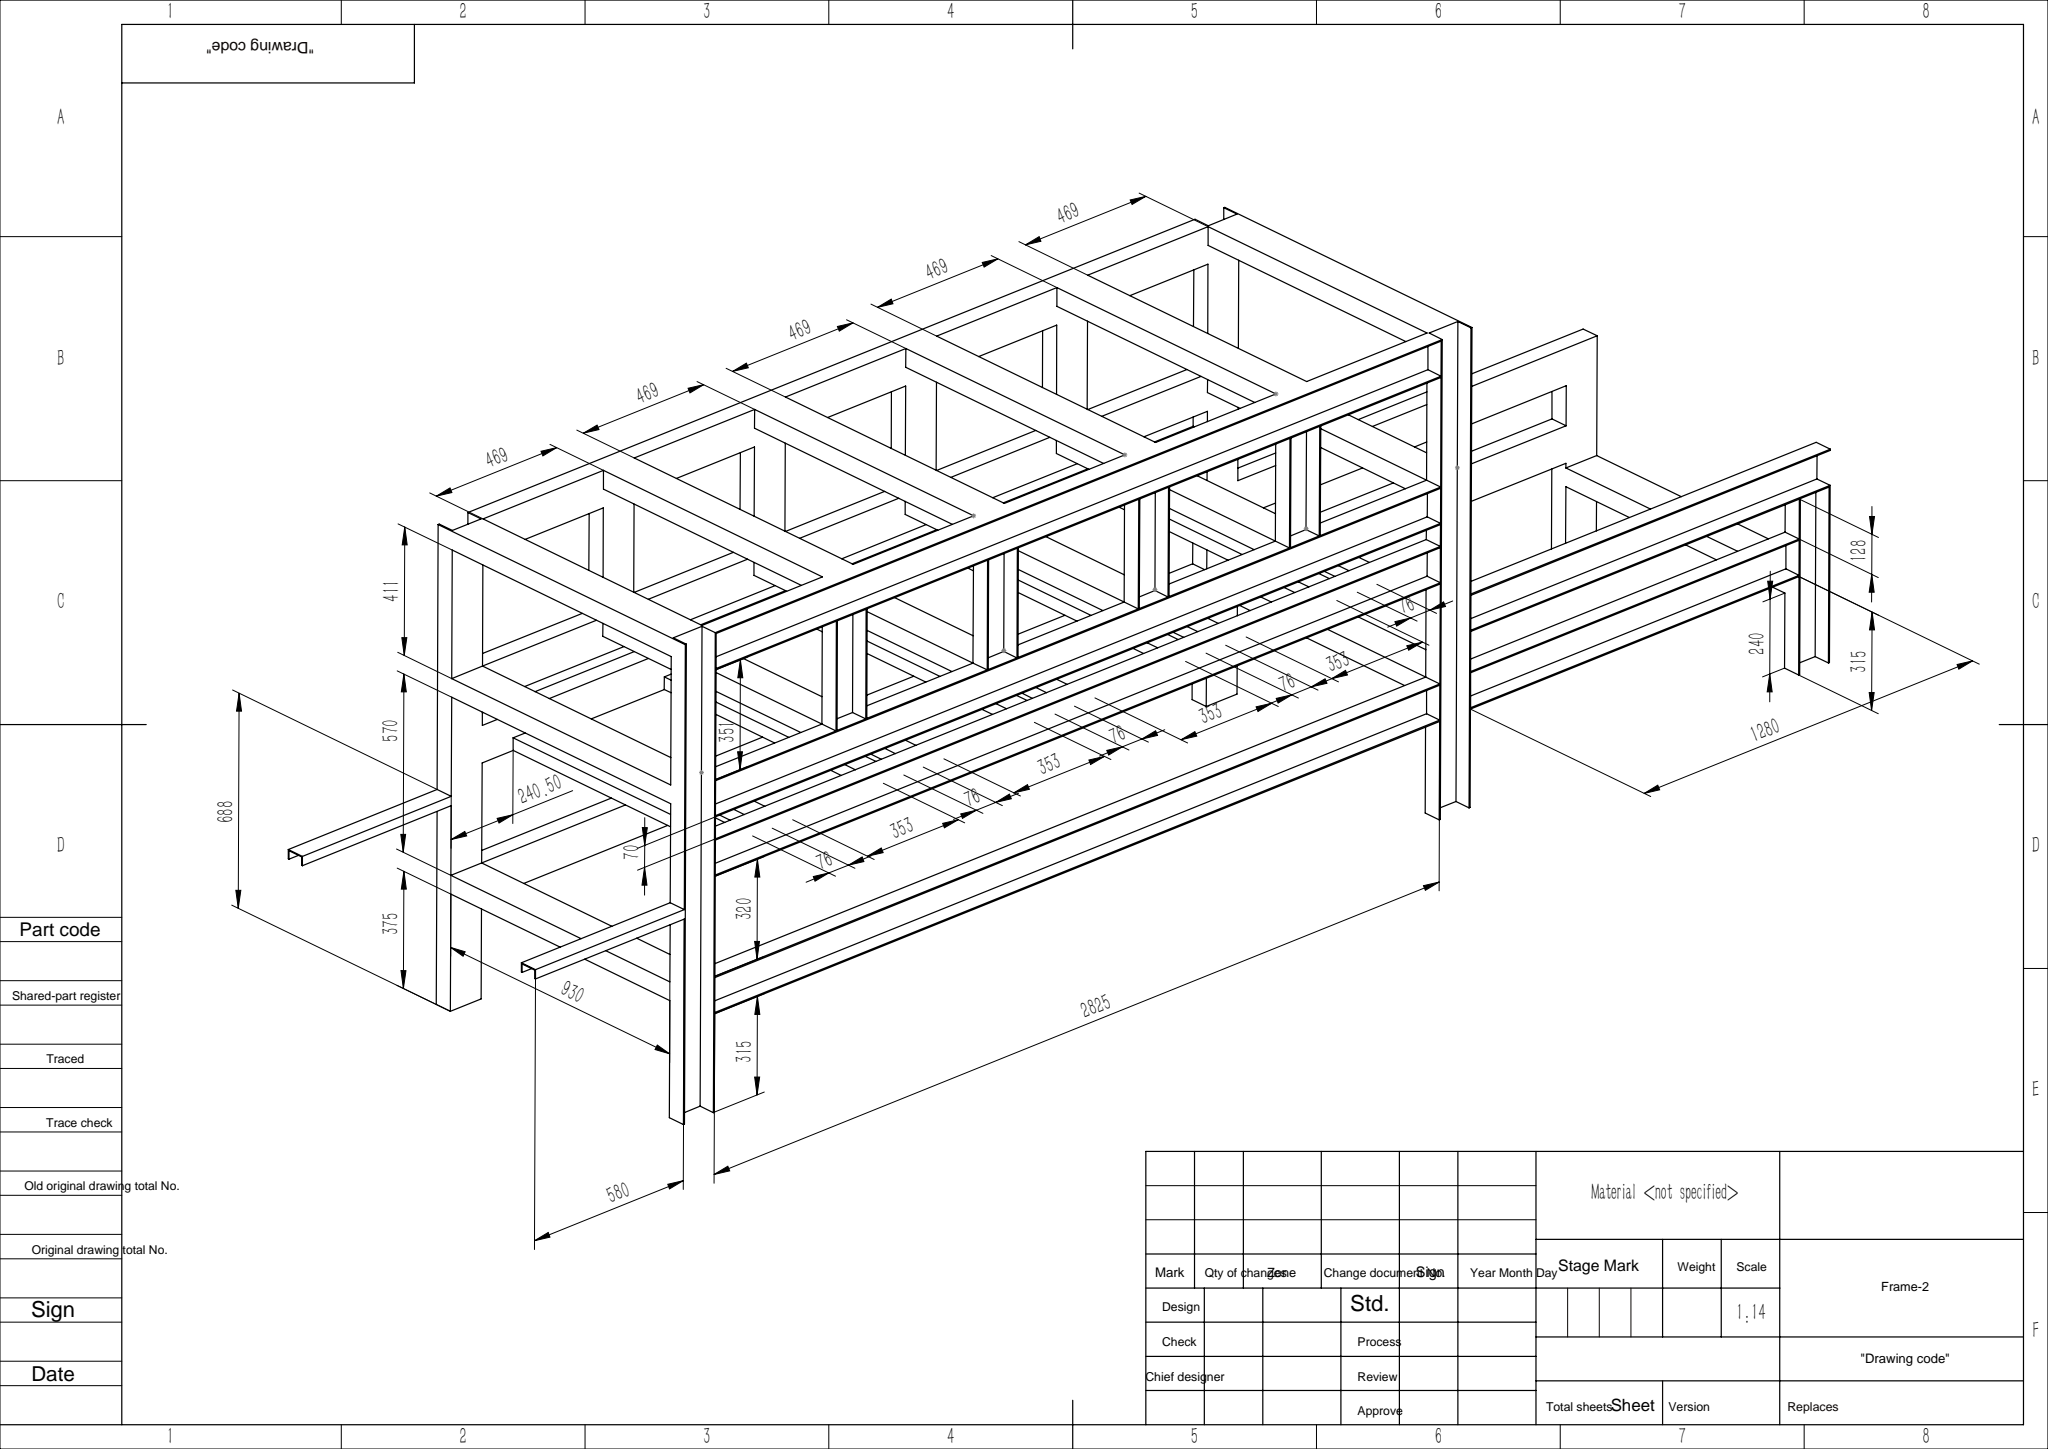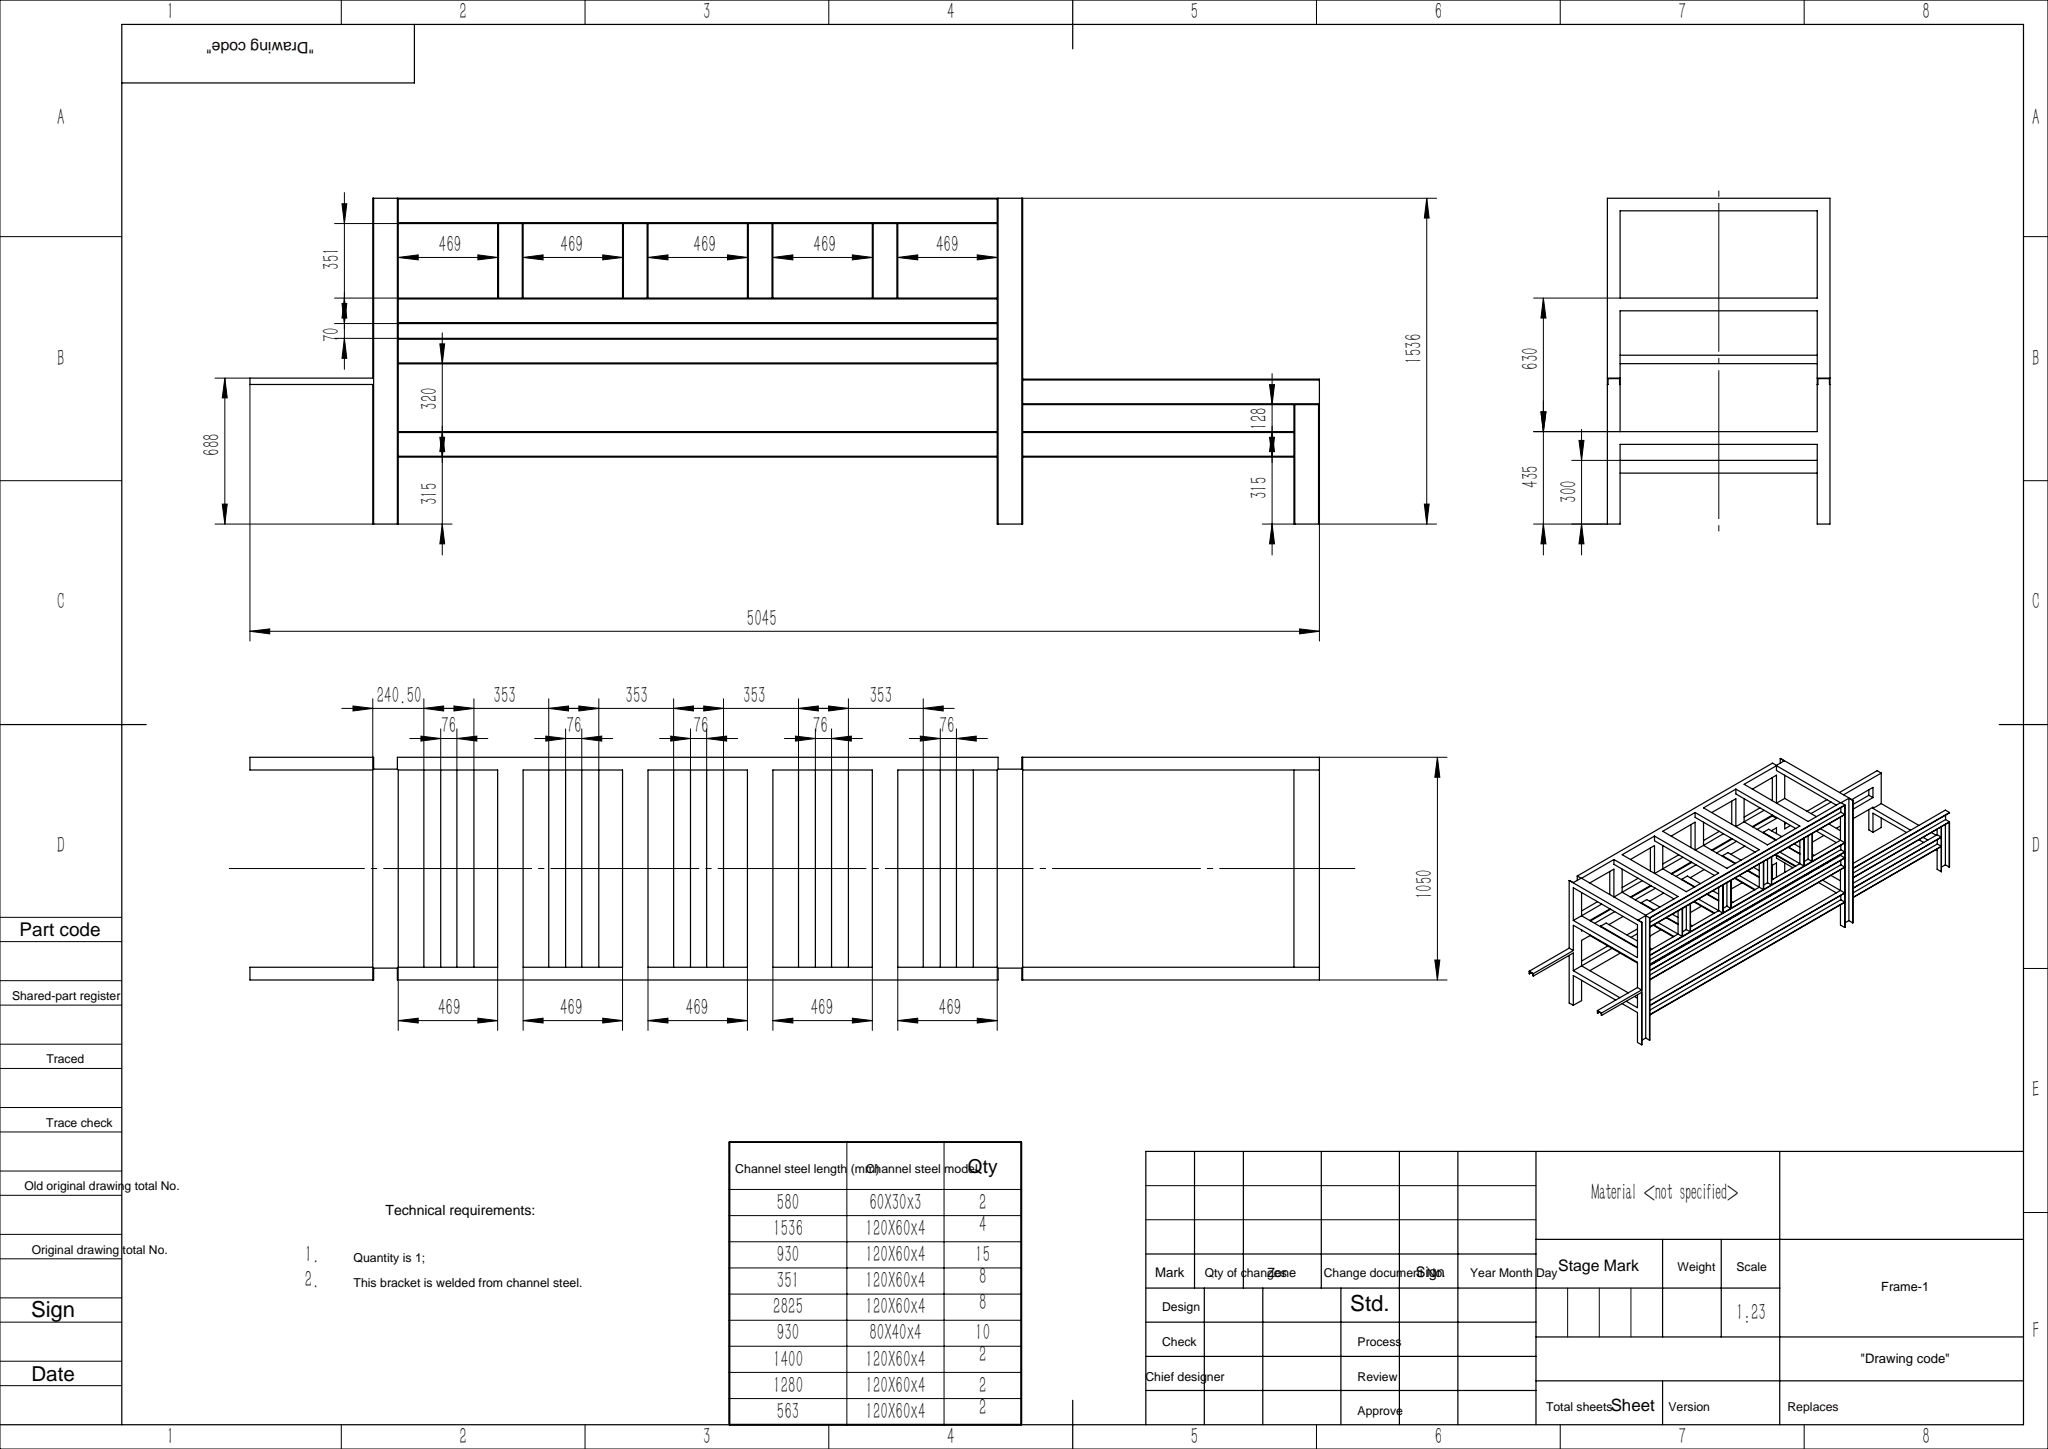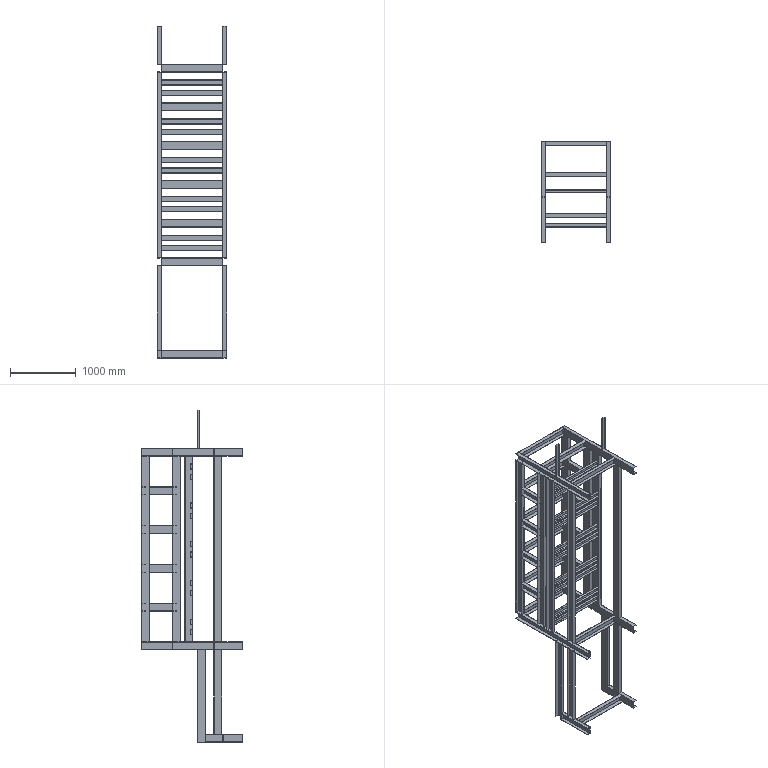Part | SolidWorks | features ICE 10, LPattern 7, SketchPattern 2, CombineBodies 1, Extrusion 1 | 1 solid | 419 faces | box 1050 x 1536 x 5045 mm | volume 54295984 mm3 | plane 419